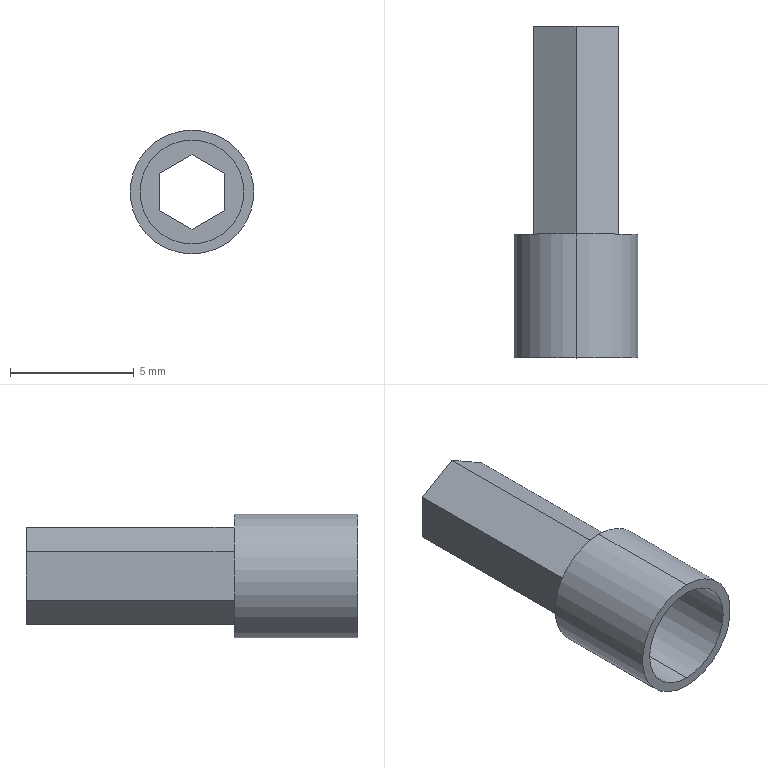Part | SolidWorks | features Extrusion 1, ICE 1, Shell 1 | 1 solid | 20 faces | box 5 x 13.4 x 5 mm | volume 67.021 mm3 | plane 16 | cylinder 4 | commonest cylinder face diameters 4.2 x2 5 x2
STEP:
#1=CARTESIAN_POINT('',(0.,4.6,-2.1));
#2=VERTEX_POINT('',#1);
#3=CARTESIAN_POINT('',(0.,4.6,2.1));
#4=VERTEX_POINT('',#3);
#5=CARTESIAN_POINT('',(0.,4.6,0.));
#6=DIRECTION('',(0.,1.,0.));
#7=DIRECTION('',(0.,0.,1.));
#8=AXIS2_PLACEMENT_3D('',#5,#6,#7);
#9=CIRCLE('',#8,2.1);
#10=EDGE_CURVE('',#2,#4,#9,.T.);
#11=ORIENTED_EDGE('',*,*,#10,.T.);
#12=CARTESIAN_POINT('',(0.,0.,2.1));
#13=VERTEX_POINT('',#12);
#14=CARTESIAN_POINT('',(0.,5.,2.1));
#15=DIRECTION('',(0.,-1.,0.));
#16=VECTOR('',#15,1000.);
#17=LINE('',#14,#16);
#18=EDGE_CURVE('',#4,#13,#17,.T.);
#19=ORIENTED_EDGE('',*,*,#18,.T.);
#20=CARTESIAN_POINT('',(0.,0.,-2.1));
#21=VERTEX_POINT('',#20);
#22=CARTESIAN_POINT('',(0.,0.,0.));
#23=DIRECTION('',(0.,1.,0.));
#24=DIRECTION('',(0.,0.,1.));
#25=AXIS2_PLACEMENT_3D('',#22,#23,#24);
#26=CIRCLE('',#25,2.1);
#27=EDGE_CURVE('',#21,#13,#26,.T.);
#28=ORIENTED_EDGE('',*,*,#27,.F.);
#29=CARTESIAN_POINT('',(0.,5.,-2.1));
#30=DIRECTION('',(0.,-1.,0.));
#31=VECTOR('',#30,1000.);
#32=LINE('',#29,#31);
#33=EDGE_CURVE('',#2,#21,#32,.T.);
#34=ORIENTED_EDGE('',*,*,#33,.F.);
#35=EDGE_LOOP('',(#11,#19,#28,#34));
#36=FACE_OUTER_BOUND('',#35,.T.);
#37=CARTESIAN_POINT('',(0.,5.,0.));
#38=DIRECTION('',(0.,-1.,0.));
#39=DIRECTION('',(0.,0.,-1.));
#40=AXIS2_PLACEMENT_3D('',#37,#38,#39);
#41=CYLINDRICAL_SURFACE('',#40,2.1);
#42=ADVANCED_FACE('',(#36),#41,.F.);
#43=CARTESIAN_POINT('',(0.,5.,2.5));
#44=VERTEX_POINT('',#43);
#45=CARTESIAN_POINT('',(0.,5.,-2.5));
#46=VERTEX_POINT('',#45);
#47=CARTESIAN_POINT('',(0.,5.,0.));
#48=DIRECTION('',(0.,1.,0.));
#49=DIRECTION('',(0.,0.,1.));
#50=AXIS2_PLACEMENT_3D('',#47,#48,#49);
#51=CIRCLE('',#50,2.5);
#52=EDGE_CURVE('',#44,#46,#51,.T.);
#53=ORIENTED_EDGE('',*,*,#52,.F.);
#54=CARTESIAN_POINT('',(0.,0.,2.5));
#55=VERTEX_POINT('',#54);
#56=CARTESIAN_POINT('',(0.,5.,2.5));
#57=DIRECTION('',(0.,-1.,0.));
#58=VECTOR('',#57,1000.);
#59=LINE('',#56,#58);
#60=EDGE_CURVE('',#44,#55,#59,.T.);
#61=ORIENTED_EDGE('',*,*,#60,.T.);
#62=CARTESIAN_POINT('',(0.,0.,-2.5));
#63=VERTEX_POINT('',#62);
#64=CARTESIAN_POINT('',(0.,0.,0.));
#65=DIRECTION('',(0.,1.,0.));
#66=DIRECTION('',(0.,0.,1.));
#67=AXIS2_PLACEMENT_3D('',#64,#65,#66);
#68=CIRCLE('',#67,2.5);
#69=EDGE_CURVE('',#55,#63,#68,.T.);
#70=ORIENTED_EDGE('',*,*,#69,.T.);
#71=CARTESIAN_POINT('',(0.,5.,-2.5));
#72=DIRECTION('',(0.,-1.,0.));
#73=VECTOR('',#72,1000.);
#74=LINE('',#71,#73);
#75=EDGE_CURVE('',#46,#63,#74,.T.);
#76=ORIENTED_EDGE('',*,*,#75,.F.);
#77=EDGE_LOOP('',(#53,#61,#70,#76));
#78=FACE_OUTER_BOUND('',#77,.T.);
#79=CARTESIAN_POINT('',(0.,5.,0.));
#80=DIRECTION('',(0.,-1.,0.));
#81=DIRECTION('',(0.,0.,-1.));
#82=AXIS2_PLACEMENT_3D('',#79,#80,#81);
#83=CYLINDRICAL_SURFACE('',#82,2.5);
#84=ADVANCED_FACE('',(#78),#83,.T.);
#85=ORIENTED_EDGE('',*,*,#60,.F.);
#86=CARTESIAN_POINT('',(0.,5.,0.));
#87=DIRECTION('',(0.,1.,0.));
#88=DIRECTION('',(0.,0.,1.));
#89=AXIS2_PLACEMENT_3D('',#86,#87,#88);
#90=CIRCLE('',#89,2.5);
#91=EDGE_CURVE('',#46,#44,#90,.T.);
#92=ORIENTED_EDGE('',*,*,#91,.F.);
#93=ORIENTED_EDGE('',*,*,#75,.T.);
#94=CARTESIAN_POINT('',(0.,0.,0.));
#95=DIRECTION('',(0.,1.,0.));
#96=DIRECTION('',(0.,0.,1.));
#97=AXIS2_PLACEMENT_3D('',#94,#95,#96);
#98=CIRCLE('',#97,2.5);
#99=EDGE_CURVE('',#63,#55,#98,.T.);
#100=ORIENTED_EDGE('',*,*,#99,.T.);
#101=EDGE_LOOP('',(#85,#92,#93,#100));
#102=FACE_OUTER_BOUND('',#101,.T.);
#103=CARTESIAN_POINT('',(0.,5.,0.));
#104=DIRECTION('',(0.,-1.,0.));
#105=DIRECTION('',(0.,0.,-1.));
#106=AXIS2_PLACEMENT_3D('',#103,#104,#105);
#107=CYLINDRICAL_SURFACE('',#106,2.5);
#108=ADVANCED_FACE('',(#102),#107,.T.);
#109=CARTESIAN_POINT('',(0.,5.,-1.963));
#110=VERTEX_POINT('',#109);
#111=CARTESIAN_POINT('',(1.7,5.,-0.9815));
#112=VERTEX_POINT('',#111);
#113=CARTESIAN_POINT('',(1.7,5.,-0.9815));
#114=DIRECTION('',(0.866,0.,0.5));
#115=VECTOR('',#114,1000.);
#116=LINE('',#113,#115);
#117=EDGE_CURVE('',#110,#112,#116,.T.);
#118=ORIENTED_EDGE('',*,*,#117,.T.);
#119=CARTESIAN_POINT('',(1.7,5.,0.9815));
#120=VERTEX_POINT('',#119);
#121=CARTESIAN_POINT('',(1.7,5.,0.9815));
#122=DIRECTION('',(0.,0.,1.));
#123=VECTOR('',#122,1000.);
#124=LINE('',#121,#123);
#125=EDGE_CURVE('',#112,#120,#124,.T.);
#126=ORIENTED_EDGE('',*,*,#125,.T.);
#127=CARTESIAN_POINT('',(0.,5.,1.963));
#128=VERTEX_POINT('',#127);
#129=CARTESIAN_POINT('',(0.,5.,1.963));
#130=DIRECTION('',(-0.866,0.,0.5));
#131=VECTOR('',#130,1000.);
#132=LINE('',#129,#131);
#133=EDGE_CURVE('',#120,#128,#132,.T.);
#134=ORIENTED_EDGE('',*,*,#133,.T.);
#135=CARTESIAN_POINT('',(-1.7,5.,0.9815));
#136=VERTEX_POINT('',#135);
#137=CARTESIAN_POINT('',(-1.7,5.,0.9815));
#138=DIRECTION('',(-0.866,0.,-0.5));
#139=VECTOR('',#138,1000.);
#140=LINE('',#137,#139);
#141=EDGE_CURVE('',#128,#136,#140,.T.);
#142=ORIENTED_EDGE('',*,*,#141,.T.);
#143=CARTESIAN_POINT('',(-1.7,5.,-0.9815));
#144=VERTEX_POINT('',#143);
#145=CARTESIAN_POINT('',(-1.7,5.,-0.9815));
#146=DIRECTION('',(0.,0.,-1.));
#147=VECTOR('',#146,1000.);
#148=LINE('',#145,#147);
#149=EDGE_CURVE('',#136,#144,#148,.T.);
#150=ORIENTED_EDGE('',*,*,#149,.T.);
#151=CARTESIAN_POINT('',(0.,5.,-1.963));
#152=DIRECTION('',(0.866,0.,-0.5));
#153=VECTOR('',#152,1000.);
#154=LINE('',#151,#153);
#155=EDGE_CURVE('',#144,#110,#154,.T.);
#156=ORIENTED_EDGE('',*,*,#155,.T.);
#157=EDGE_LOOP('',(#118,#126,#134,#142,#150,#156));
#158=FACE_BOUND('',#157,.T.);
#159=ORIENTED_EDGE('',*,*,#91,.T.);
#160=ORIENTED_EDGE('',*,*,#52,.T.);
#161=EDGE_LOOP('',(#159,#160));
#162=FACE_OUTER_BOUND('',#161,.T.);
#163=CARTESIAN_POINT('',(0.,5.,0.));
#164=DIRECTION('',(0.,1.,0.));
#165=DIRECTION('',(0.,0.,1.));
#166=AXIS2_PLACEMENT_3D('',#163,#164,#165);
#167=PLANE('',#166);
#168=ADVANCED_FACE('',(#158,#162),#167,.T.);
#169=ORIENTED_EDGE('',*,*,#27,.T.);
#170=CARTESIAN_POINT('',(0.,0.,0.));
#171=DIRECTION('',(0.,1.,0.));
#172=DIRECTION('',(0.,0.,1.));
#173=AXIS2_PLACEMENT_3D('',#170,#171,#172);
#174=CIRCLE('',#173,2.1);
#175=EDGE_CURVE('',#13,#21,#174,.T.);
#176=ORIENTED_EDGE('',*,*,#175,.T.);
#177=EDGE_LOOP('',(#169,#176));
#178=FACE_BOUND('',#177,.T.);
#179=ORIENTED_EDGE('',*,*,#99,.F.);
#180=ORIENTED_EDGE('',*,*,#69,.F.);
#181=EDGE_LOOP('',(#179,#180));
#182=FACE_OUTER_BOUND('',#181,.T.);
#183=CARTESIAN_POINT('',(0.,0.,0.));
#184=DIRECTION('',(0.,1.,0.));
#185=DIRECTION('',(0.,0.,1.));
#186=AXIS2_PLACEMENT_3D('',#183,#184,#185);
#187=PLANE('',#186);
#188=ADVANCED_FACE('',(#178,#182),#187,.F.);
#189=ORIENTED_EDGE('',*,*,#117,.F.);
#190=CARTESIAN_POINT('',(0.,13.4,-1.963));
#191=VERTEX_POINT('',#190);
#192=CARTESIAN_POINT('',(0.,-0.1936,-1.963));
#193=DIRECTION('',(0.,1.,0.));
#194=VECTOR('',#193,1000.);
#195=LINE('',#192,#194);
#196=EDGE_CURVE('',#110,#191,#195,.T.);
#197=ORIENTED_EDGE('',*,*,#196,.T.);
#198=CARTESIAN_POINT('',(1.7,13.4,-0.9815));
#199=VERTEX_POINT('',#198);
#200=CARTESIAN_POINT('',(1.7,13.4,-0.9815));
#201=DIRECTION('',(-0.866,0.,-0.5));
#202=VECTOR('',#201,1000.);
#203=LINE('',#200,#202);
#204=EDGE_CURVE('',#199,#191,#203,.T.);
#205=ORIENTED_EDGE('',*,*,#204,.F.);
#206=CARTESIAN_POINT('',(1.7,-0.1936,-0.9815));
#207=DIRECTION('',(0.,1.,0.));
#208=VECTOR('',#207,1000.);
#209=LINE('',#206,#208);
#210=EDGE_CURVE('',#112,#199,#209,.T.);
#211=ORIENTED_EDGE('',*,*,#210,.F.);
#212=EDGE_LOOP('',(#189,#197,#205,#211));
#213=FACE_OUTER_BOUND('',#212,.T.);
#214=CARTESIAN_POINT('',(1.7,-0.1936,-0.9815));
#215=DIRECTION('',(0.5,0.,-0.866));
#216=DIRECTION('',(-0.866,0.,-0.5));
#217=AXIS2_PLACEMENT_3D('',#214,#215,#216);
#218=PLANE('',#217);
#219=ADVANCED_FACE('',(#213),#218,.T.);
#220=ORIENTED_EDGE('',*,*,#125,.F.);
#221=ORIENTED_EDGE('',*,*,#210,.T.);
#222=CARTESIAN_POINT('',(1.7,13.4,0.9815));
#223=VERTEX_POINT('',#222);
#224=CARTESIAN_POINT('',(1.7,13.4,0.9815));
#225=DIRECTION('',(0.,0.,-1.));
#226=VECTOR('',#225,1000.);
#227=LINE('',#224,#226);
#228=EDGE_CURVE('',#223,#199,#227,.T.);
#229=ORIENTED_EDGE('',*,*,#228,.F.);
#230=CARTESIAN_POINT('',(1.7,-0.1936,0.9815));
#231=DIRECTION('',(0.,1.,0.));
#232=VECTOR('',#231,1000.);
#233=LINE('',#230,#232);
#234=EDGE_CURVE('',#120,#223,#233,.T.);
#235=ORIENTED_EDGE('',*,*,#234,.F.);
#236=EDGE_LOOP('',(#220,#221,#229,#235));
#237=FACE_OUTER_BOUND('',#236,.T.);
#238=CARTESIAN_POINT('',(1.7,-0.1936,0.9815));
#239=DIRECTION('',(1.,0.,0.));
#240=DIRECTION('',(0.,0.,-1.));
#241=AXIS2_PLACEMENT_3D('',#238,#239,#240);
#242=PLANE('',#241);
#243=ADVANCED_FACE('',(#237),#242,.T.);
#244=ORIENTED_EDGE('',*,*,#133,.F.);
#245=ORIENTED_EDGE('',*,*,#234,.T.);
#246=CARTESIAN_POINT('',(0.,13.4,1.963));
#247=VERTEX_POINT('',#246);
#248=CARTESIAN_POINT('',(0.,13.4,1.963));
#249=DIRECTION('',(0.866,0.,-0.5));
#250=VECTOR('',#249,1000.);
#251=LINE('',#248,#250);
#252=EDGE_CURVE('',#247,#223,#251,.T.);
#253=ORIENTED_EDGE('',*,*,#252,.F.);
#254=CARTESIAN_POINT('',(0.,-0.1936,1.963));
#255=DIRECTION('',(0.,1.,0.));
#256=VECTOR('',#255,1000.);
#257=LINE('',#254,#256);
#258=EDGE_CURVE('',#128,#247,#257,.T.);
#259=ORIENTED_EDGE('',*,*,#258,.F.);
#260=EDGE_LOOP('',(#244,#245,#253,#259));
#261=FACE_OUTER_BOUND('',#260,.T.);
#262=CARTESIAN_POINT('',(0.,-0.1936,1.963));
#263=DIRECTION('',(0.5,0.,0.866));
#264=DIRECTION('',(0.866,0.,-0.5));
#265=AXIS2_PLACEMENT_3D('',#262,#263,#264);
#266=PLANE('',#265);
#267=ADVANCED_FACE('',(#261),#266,.T.);
#268=ORIENTED_EDGE('',*,*,#141,.F.);
#269=ORIENTED_EDGE('',*,*,#258,.T.);
#270=CARTESIAN_POINT('',(-1.7,13.4,0.9815));
#271=VERTEX_POINT('',#270);
#272=CARTESIAN_POINT('',(-1.7,13.4,0.9815));
#273=DIRECTION('',(0.866,0.,0.5));
#274=VECTOR('',#273,1000.);
#275=LINE('',#272,#274);
#276=EDGE_CURVE('',#271,#247,#275,.T.);
#277=ORIENTED_EDGE('',*,*,#276,.F.);
#278=CARTESIAN_POINT('',(-1.7,-0.1936,0.9815));
#279=DIRECTION('',(0.,1.,0.));
#280=VECTOR('',#279,1000.);
#281=LINE('',#278,#280);
#282=EDGE_CURVE('',#136,#271,#281,.T.);
#283=ORIENTED_EDGE('',*,*,#282,.F.);
#284=EDGE_LOOP('',(#268,#269,#277,#283));
#285=FACE_OUTER_BOUND('',#284,.T.);
#286=CARTESIAN_POINT('',(-1.7,-0.1936,0.9815));
#287=DIRECTION('',(-0.5,0.,0.866));
#288=DIRECTION('',(0.866,0.,0.5));
#289=AXIS2_PLACEMENT_3D('',#286,#287,#288);
#290=PLANE('',#289);
#291=ADVANCED_FACE('',(#285),#290,.T.);
#292=ORIENTED_EDGE('',*,*,#149,.F.);
#293=ORIENTED_EDGE('',*,*,#282,.T.);
#294=CARTESIAN_POINT('',(-1.7,13.4,-0.9815));
#295=VERTEX_POINT('',#294);
#296=CARTESIAN_POINT('',(-1.7,13.4,-0.9815));
#297=DIRECTION('',(0.,0.,1.));
#298=VECTOR('',#297,1000.);
#299=LINE('',#296,#298);
#300=EDGE_CURVE('',#295,#271,#299,.T.);
#301=ORIENTED_EDGE('',*,*,#300,.F.);
#302=CARTESIAN_POINT('',(-1.7,-0.1936,-0.9815));
#303=DIRECTION('',(0.,1.,0.));
#304=VECTOR('',#303,1000.);
#305=LINE('',#302,#304);
#306=EDGE_CURVE('',#144,#295,#305,.T.);
#307=ORIENTED_EDGE('',*,*,#306,.F.);
#308=EDGE_LOOP('',(#292,#293,#301,#307));
#309=FACE_OUTER_BOUND('',#308,.T.);
#310=CARTESIAN_POINT('',(-1.7,-0.1936,-0.9815));
#311=DIRECTION('',(-1.,0.,0.));
#312=DIRECTION('',(0.,0.,1.));
#313=AXIS2_PLACEMENT_3D('',#310,#311,#312);
#314=PLANE('',#313);
#315=ADVANCED_FACE('',(#309),#314,.T.);
#316=ORIENTED_EDGE('',*,*,#155,.F.);
#317=ORIENTED_EDGE('',*,*,#306,.T.);
#318=CARTESIAN_POINT('',(0.,13.4,-1.963));
#319=DIRECTION('',(-0.866,0.,0.5));
#320=VECTOR('',#319,1000.);
#321=LINE('',#318,#320);
#322=EDGE_CURVE('',#191,#295,#321,.T.);
#323=ORIENTED_EDGE('',*,*,#322,.F.);
#324=ORIENTED_EDGE('',*,*,#196,.F.);
#325=EDGE_LOOP('',(#316,#317,#323,#324));
#326=FACE_OUTER_BOUND('',#325,.T.);
#327=CARTESIAN_POINT('',(0.,-0.1936,-1.963));
#328=DIRECTION('',(-0.5,0.,-0.866));
#329=DIRECTION('',(-0.866,0.,0.5));
#330=AXIS2_PLACEMENT_3D('',#327,#328,#329);
#331=PLANE('',#330);
#332=ADVANCED_FACE('',(#326),#331,.T.);
#333=CARTESIAN_POINT('',(1.3,13.4,-0.7506));
#334=VERTEX_POINT('',#333);
#335=CARTESIAN_POINT('',(0.,13.4,-1.501));
#336=VERTEX_POINT('',#335);
#337=CARTESIAN_POINT('',(0.65,13.4,-1.126));
#338=DIRECTION('',(-0.866,0.,-0.5));
#339=VECTOR('',#338,1000.);
#340=LINE('',#337,#339);
#341=EDGE_CURVE('',#334,#336,#340,.T.);
#342=ORIENTED_EDGE('',*,*,#341,.F.);
#343=CARTESIAN_POINT('',(1.3,13.4,0.7506));
#344=VERTEX_POINT('',#343);
#345=CARTESIAN_POINT('',(1.3,13.4,0.));
#346=DIRECTION('',(0.,0.,-1.));
#347=VECTOR('',#346,1000.);
#348=LINE('',#345,#347);
#349=EDGE_CURVE('',#344,#334,#348,.T.);
#350=ORIENTED_EDGE('',*,*,#349,.F.);
#351=CARTESIAN_POINT('',(0.,13.4,1.501));
#352=VERTEX_POINT('',#351);
#353=CARTESIAN_POINT('',(0.65,13.4,1.126));
#354=DIRECTION('',(0.866,0.,-0.5));
#355=VECTOR('',#354,1000.);
#356=LINE('',#353,#355);
#357=EDGE_CURVE('',#352,#344,#356,.T.);
#358=ORIENTED_EDGE('',*,*,#357,.F.);
#359=CARTESIAN_POINT('',(-1.3,13.4,0.7506));
#360=VERTEX_POINT('',#359);
#361=CARTESIAN_POINT('',(-0.65,13.4,1.126));
#362=DIRECTION('',(0.866,0.,0.5));
#363=VECTOR('',#362,1000.);
#364=LINE('',#361,#363);
#365=EDGE_CURVE('',#360,#352,#364,.T.);
#366=ORIENTED_EDGE('',*,*,#365,.F.);
#367=CARTESIAN_POINT('',(-1.3,13.4,-0.7506));
#368=VERTEX_POINT('',#367);
#369=CARTESIAN_POINT('',(-1.3,13.4,0.));
#370=DIRECTION('',(0.,0.,1.));
#371=VECTOR('',#370,1000.);
#372=LINE('',#369,#371);
#373=EDGE_CURVE('',#368,#360,#372,.T.);
#374=ORIENTED_EDGE('',*,*,#373,.F.);
#375=CARTESIAN_POINT('',(-0.65,13.4,-1.126));
#376=DIRECTION('',(-0.866,0.,0.5));
#377=VECTOR('',#376,1000.);
#378=LINE('',#375,#377);
#379=EDGE_CURVE('',#336,#368,#378,.T.);
#380=ORIENTED_EDGE('',*,*,#379,.F.);
#381=EDGE_LOOP('',(#342,#350,#358,#366,#374,#380));
#382=FACE_BOUND('',#381,.T.);
#383=ORIENTED_EDGE('',*,*,#204,.T.);
#384=ORIENTED_EDGE('',*,*,#322,.T.);
#385=ORIENTED_EDGE('',*,*,#300,.T.);
#386=ORIENTED_EDGE('',*,*,#276,.T.);
#387=ORIENTED_EDGE('',*,*,#252,.T.);
#388=ORIENTED_EDGE('',*,*,#228,.T.);
#389=EDGE_LOOP('',(#383,#384,#385,#386,#387,#388));
#390=FACE_OUTER_BOUND('',#389,.T.);
#391=CARTESIAN_POINT('',(0.,13.4,0.));
#392=DIRECTION('',(0.,1.,0.));
#393=DIRECTION('',(0.,0.,1.));
#394=AXIS2_PLACEMENT_3D('',#391,#392,#393);
#395=PLANE('',#394);
#396=ADVANCED_FACE('',(#382,#390),#395,.T.);
#397=ORIENTED_EDGE('',*,*,#18,.F.);
#398=CARTESIAN_POINT('',(0.,4.6,0.));
#399=DIRECTION('',(0.,1.,0.));
#400=DIRECTION('',(0.,0.,1.));
#401=AXIS2_PLACEMENT_3D('',#398,#399,#400);
#402=CIRCLE('',#401,2.1);
#403=EDGE_CURVE('',#4,#2,#402,.T.);
#404=ORIENTED_EDGE('',*,*,#403,.T.);
#405=ORIENTED_EDGE('',*,*,#33,.T.);
#406=ORIENTED_EDGE('',*,*,#175,.F.);
#407=EDGE_LOOP('',(#397,#404,#405,#406));
#408=FACE_OUTER_BOUND('',#407,.T.);
#409=CARTESIAN_POINT('',(0.,5.,0.));
#410=DIRECTION('',(0.,-1.,0.));
#411=DIRECTION('',(0.,0.,-1.));
#412=AXIS2_PLACEMENT_3D('',#409,#410,#411);
#413=CYLINDRICAL_SURFACE('',#412,2.1);
#414=ADVANCED_FACE('',(#408),#413,.F.);
#415=CARTESIAN_POINT('',(0.,4.6,-1.501));
#416=VERTEX_POINT('',#415);
#417=CARTESIAN_POINT('',(1.3,4.6,-0.7506));
#418=VERTEX_POINT('',#417);
#419=CARTESIAN_POINT('',(1.5,4.6,-0.6351));
#420=DIRECTION('',(0.866,0.,0.5));
#421=VECTOR('',#420,1000.);
#422=LINE('',#419,#421);
#423=EDGE_CURVE('',#416,#418,#422,.T.);
#424=ORIENTED_EDGE('',*,*,#423,.F.);
#425=CARTESIAN_POINT('',(-1.3,4.6,-0.7506));
#426=VERTEX_POINT('',#425);
#427=CARTESIAN_POINT('',(0.2,4.6,-1.617));
#428=DIRECTION('',(0.866,0.,-0.5));
#429=VECTOR('',#428,1000.);
#430=LINE('',#427,#429);
#431=EDGE_CURVE('',#426,#416,#430,.T.);
#432=ORIENTED_EDGE('',*,*,#431,.F.);
#433=CARTESIAN_POINT('',(-1.3,4.6,0.7506));
#434=VERTEX_POINT('',#433);
#435=CARTESIAN_POINT('',(-1.3,4.6,-0.9815));
#436=DIRECTION('',(0.,0.,-1.));
#437=VECTOR('',#436,1000.);
#438=LINE('',#435,#437);
#439=EDGE_CURVE('',#434,#426,#438,.T.);
#440=ORIENTED_EDGE('',*,*,#439,.F.);
#441=CARTESIAN_POINT('',(0.,4.6,1.501));
#442=VERTEX_POINT('',#441);
#443=CARTESIAN_POINT('',(-1.5,4.6,0.6351));
#444=DIRECTION('',(-0.866,0.,-0.5));
#445=VECTOR('',#444,1000.);
#446=LINE('',#443,#445);
#447=EDGE_CURVE('',#442,#434,#446,.T.);
#448=ORIENTED_EDGE('',*,*,#447,.F.);
#449=CARTESIAN_POINT('',(1.3,4.6,0.7506));
#450=VERTEX_POINT('',#449);
#451=CARTESIAN_POINT('',(-0.2,4.6,1.617));
#452=DIRECTION('',(-0.866,0.,0.5));
#453=VECTOR('',#452,1000.);
#454=LINE('',#451,#453);
#455=EDGE_CURVE('',#450,#442,#454,.T.);
#456=ORIENTED_EDGE('',*,*,#455,.F.);
#457=CARTESIAN_POINT('',(1.3,4.6,0.9815));
#458=DIRECTION('',(0.,0.,1.));
#459=VECTOR('',#458,1000.);
#460=LINE('',#457,#459);
#461=EDGE_CURVE('',#418,#450,#460,.T.);
#462=ORIENTED_EDGE('',*,*,#461,.F.);
#463=EDGE_LOOP('',(#424,#432,#440,#448,#456,#462));
#464=FACE_BOUND('',#463,.T.);
#465=ORIENTED_EDGE('',*,*,#10,.F.);
#466=ORIENTED_EDGE('',*,*,#403,.F.);
#467=EDGE_LOOP('',(#465,#466));
#468=FACE_OUTER_BOUND('',#467,.T.);
#469=CARTESIAN_POINT('',(0.,4.6,0.));
#470=DIRECTION('',(0.,1.,0.));
#471=DIRECTION('',(0.,0.,1.));
#472=AXIS2_PLACEMENT_3D('',#469,#470,#471);
#473=PLANE('',#472);
#474=ADVANCED_FACE('',(#464,#468),#473,.F.);
#475=ORIENTED_EDGE('',*,*,#423,.T.);
#476=CARTESIAN_POINT('',(1.3,-0.1936,-0.7506));
#477=DIRECTION('',(0.,1.,0.));
#478=VECTOR('',#477,1000.);
#479=LINE('',#476,#478);
#480=EDGE_CURVE('',#418,#334,#479,.T.);
#481=ORIENTED_EDGE('',*,*,#480,.T.);
#482=ORIENTED_EDGE('',*,*,#341,.T.);
#483=CARTESIAN_POINT('',(0.,-0.1936,-1.501));
#484=DIRECTION('',(0.,1.,0.));
#485=VECTOR('',#484,1000.);
#486=LINE('',#483,#485);
#487=EDGE_CURVE('',#416,#336,#486,.T.);
#488=ORIENTED_EDGE('',*,*,#487,.F.);
#489=EDGE_LOOP('',(#475,#481,#482,#488));
#490=FACE_OUTER_BOUND('',#489,.T.);
#491=CARTESIAN_POINT('',(1.5,-0.1936,-0.6351));
#492=DIRECTION('',(0.5,0.,-0.866));
#493=DIRECTION('',(-0.866,0.,-0.5));
#494=AXIS2_PLACEMENT_3D('',#491,#492,#493);
#495=PLANE('',#494);
#496=ADVANCED_FACE('',(#490),#495,.F.);
#497=ORIENTED_EDGE('',*,*,#461,.T.);
#498=CARTESIAN_POINT('',(1.3,-0.1936,0.7506));
#499=DIRECTION('',(0.,1.,0.));
#500=VECTOR('',#499,1000.);
#501=LINE('',#498,#500);
#502=EDGE_CURVE('',#450,#344,#501,.T.);
#503=ORIENTED_EDGE('',*,*,#502,.T.);
#504=ORIENTED_EDGE('',*,*,#349,.T.);
#505=ORIENTED_EDGE('',*,*,#480,.F.);
#506=EDGE_LOOP('',(#497,#503,#504,#505));
#507=FACE_OUTER_BOUND('',#506,.T.);
#508=CARTESIAN_POINT('',(1.3,-0.1936,0.9815));
#509=DIRECTION('',(1.,0.,0.));
#510=DIRECTION('',(0.,0.,-1.));
#511=AXIS2_PLACEMENT_3D('',#508,#509,#510);
#512=PLANE('',#511);
#513=ADVANCED_FACE('',(#507),#512,.F.);
#514=ORIENTED_EDGE('',*,*,#455,.T.);
#515=CARTESIAN_POINT('',(0.,-0.1936,1.501));
#516=DIRECTION('',(0.,1.,0.));
#517=VECTOR('',#516,1000.);
#518=LINE('',#515,#517);
#519=EDGE_CURVE('',#442,#352,#518,.T.);
#520=ORIENTED_EDGE('',*,*,#519,.T.);
#521=ORIENTED_EDGE('',*,*,#357,.T.);
#522=ORIENTED_EDGE('',*,*,#502,.F.);
#523=EDGE_LOOP('',(#514,#520,#521,#522));
#524=FACE_OUTER_BOUND('',#523,.T.);
#525=CARTESIAN_POINT('',(-0.2,-0.1936,1.617));
#526=DIRECTION('',(0.5,0.,0.866));
#527=DIRECTION('',(0.866,0.,-0.5));
#528=AXIS2_PLACEMENT_3D('',#525,#526,#527);
#529=PLANE('',#528);
#530=ADVANCED_FACE('',(#524),#529,.F.);
#531=ORIENTED_EDGE('',*,*,#447,.T.);
#532=CARTESIAN_POINT('',(-1.3,-0.1936,0.7506));
#533=DIRECTION('',(0.,1.,0.));
#534=VECTOR('',#533,1000.);
#535=LINE('',#532,#534);
#536=EDGE_CURVE('',#434,#360,#535,.T.);
#537=ORIENTED_EDGE('',*,*,#536,.T.);
#538=ORIENTED_EDGE('',*,*,#365,.T.);
#539=ORIENTED_EDGE('',*,*,#519,.F.);
#540=EDGE_LOOP('',(#531,#537,#538,#539));
#541=FACE_OUTER_BOUND('',#540,.T.);
#542=CARTESIAN_POINT('',(-1.5,-0.1936,0.6351));
#543=DIRECTION('',(-0.5,0.,0.866));
#544=DIRECTION('',(0.866,0.,0.5));
#545=AXIS2_PLACEMENT_3D('',#542,#543,#544);
#546=PLANE('',#545);
#547=ADVANCED_FACE('',(#541),#546,.F.);
#548=ORIENTED_EDGE('',*,*,#439,.T.);
#549=CARTESIAN_POINT('',(-1.3,-0.1936,-0.7506));
#550=DIRECTION('',(0.,1.,0.));
#551=VECTOR('',#550,1000.);
#552=LINE('',#549,#551);
#553=EDGE_CURVE('',#426,#368,#552,.T.);
#554=ORIENTED_EDGE('',*,*,#553,.T.);
#555=ORIENTED_EDGE('',*,*,#373,.T.);
#556=ORIENTED_EDGE('',*,*,#536,.F.);
#557=EDGE_LOOP('',(#548,#554,#555,#556));
#558=FACE_OUTER_BOUND('',#557,.T.);
#559=CARTESIAN_POINT('',(-1.3,-0.1936,-0.9815));
#560=DIRECTION('',(-1.,0.,0.));
#561=DIRECTION('',(0.,0.,1.));
#562=AXIS2_PLACEMENT_3D('',#559,#560,#561);
#563=PLANE('',#562);
#564=ADVANCED_FACE('',(#558),#563,.F.);
#565=ORIENTED_EDGE('',*,*,#431,.T.);
#566=ORIENTED_EDGE('',*,*,#487,.T.);
#567=ORIENTED_EDGE('',*,*,#379,.T.);
#568=ORIENTED_EDGE('',*,*,#553,.F.);
#569=EDGE_LOOP('',(#565,#566,#567,#568));
#570=FACE_OUTER_BOUND('',#569,.T.);
#571=CARTESIAN_POINT('',(0.2,-0.1936,-1.617));
#572=DIRECTION('',(-0.5,0.,-0.866));
#573=DIRECTION('',(-0.866,0.,0.5));
#574=AXIS2_PLACEMENT_3D('',#571,#572,#573);
#575=PLANE('',#574);
#576=ADVANCED_FACE('',(#570),#575,.F.);
#577=CLOSED_SHELL('',(#42,#84,#108,#168,#188,#219,#243,#267,#291,#315,#332,#396,#414,#474,#496,#513,#530,#547,#564,#576));
#578=MANIFOLD_SOLID_BREP('',#577);
#579=CARTESIAN_POINT('',(0.,0.,0.));
#580=DIRECTION('',(0.,0.,1.));
#581=DIRECTION('',(1.,0.,0.));
#582=AXIS2_PLACEMENT_3D('',#579,#580,#581);
#583=(LENGTH_UNIT()NAMED_UNIT(*)SI_UNIT(.MILLI.,.METRE.));
#584=UNCERTAINTY_MEASURE_WITH_UNIT(LENGTH_MEASURE(0.00001),#583,'','');
#585=(NAMED_UNIT(*)PLANE_ANGLE_UNIT()SI_UNIT($,.RADIAN.));
#586=(NAMED_UNIT(*)SI_UNIT($,.STERADIAN.)SOLID_ANGLE_UNIT());
#587=(GEOMETRIC_REPRESENTATION_CONTEXT(3)GLOBAL_UNCERTAINTY_ASSIGNED_CONTEXT((#584))GLOBAL_UNIT_ASSIGNED_CONTEXT((#583,#585,#586))REPRESENTATION_CONTEXT('',''));
#588=ADVANCED_BREP_SHAPE_REPRESENTATION('',(#578,#582),#587);